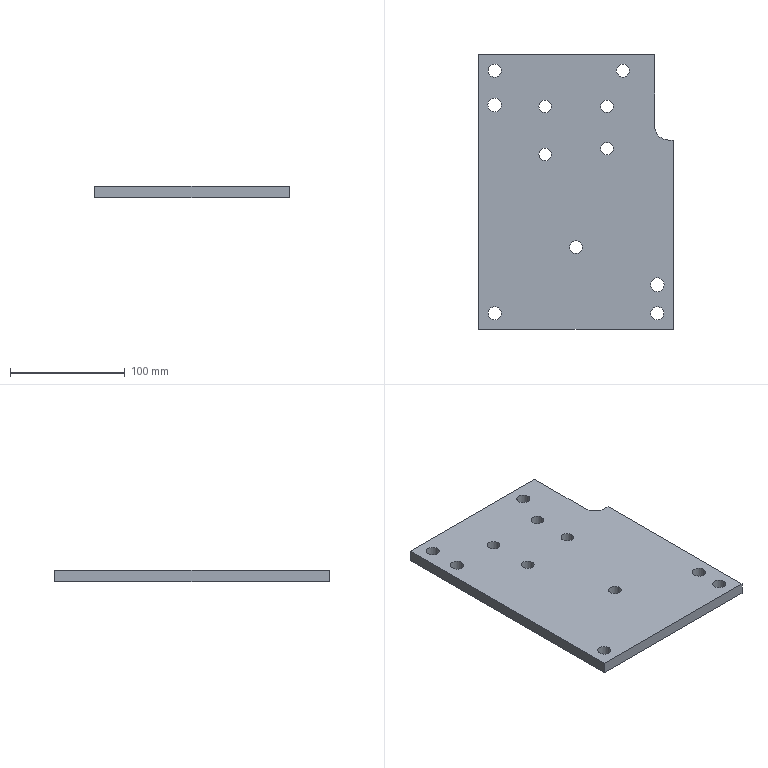Part | STEP file | lll_id2998_x_t | 1 solid | 20 faces | box 170 x 240 x 10 mm | volume 385001 mm3 | cylinder 12 | plane 8 | commonest cylinder face diameters 11 x5 11.509 x4 12 x2 24 x1
STEP:
#1=CARTESIAN_POINT('',(3581.734,-202.95,92.5));
#2=VERTEX_POINT('',#1);
#3=CARTESIAN_POINT('',(3587.234,-202.95,92.5));
#4=DIRECTION('',(0.,0.,-1.));
#5=DIRECTION('',(-1.,0.,0.));
#6=AXIS2_PLACEMENT_3D('',#3,#4,#5);
#7=CIRCLE('',#6,5.5);
#8=EDGE_CURVE('',#2,#2,#7,.T.);
#9=ORIENTED_EDGE('',*,*,#8,.F.);
#10=EDGE_LOOP('',(#9));
#11=FACE_BOUND('',#10,.T.);
#12=CARTESIAN_POINT('',(3554.876,-80.05,92.5));
#13=VERTEX_POINT('',#12);
#14=CARTESIAN_POINT('',(3560.376,-80.05,92.5));
#15=DIRECTION('',(0.,0.,1.));
#16=DIRECTION('',(-1.,0.,0.));
#17=AXIS2_PLACEMENT_3D('',#14,#15,#16);
#18=CIRCLE('',#17,5.5);
#19=EDGE_CURVE('',#13,#13,#18,.T.);
#20=ORIENTED_EDGE('',*,*,#19,.T.);
#21=EDGE_LOOP('',(#20));
#22=FACE_BOUND('',#21,.T.);
#23=CARTESIAN_POINT('',(3608.779,-80.031,92.5));
#24=VERTEX_POINT('',#23);
#25=CARTESIAN_POINT('',(3614.279,-80.031,92.5));
#26=DIRECTION('',(0.,0.,1.));
#27=DIRECTION('',(-1.,0.,0.));
#28=AXIS2_PLACEMENT_3D('',#25,#26,#27);
#29=CIRCLE('',#28,5.5);
#30=EDGE_CURVE('',#24,#24,#29,.T.);
#31=ORIENTED_EDGE('',*,*,#30,.T.);
#32=EDGE_LOOP('',(#31));
#33=FACE_BOUND('',#32,.T.);
#34=CARTESIAN_POINT('',(3510.243,-78.803,92.5));
#35=VERTEX_POINT('',#34);
#36=CARTESIAN_POINT('',(3516.243,-78.803,92.5));
#37=DIRECTION('',(0.,0.,-1.));
#38=DIRECTION('',(-1.,0.,0.));
#39=AXIS2_PLACEMENT_3D('',#36,#37,#38);
#40=CIRCLE('',#39,6.);
#41=EDGE_CURVE('',#35,#35,#40,.T.);
#42=ORIENTED_EDGE('',*,*,#41,.F.);
#43=EDGE_LOOP('',(#42));
#44=FACE_BOUND('',#43,.T.);
#45=CARTESIAN_POINT('',(3622.489,-48.803,92.5));
#46=VERTEX_POINT('',#45);
#47=CARTESIAN_POINT('',(3628.243,-48.803,92.5));
#48=DIRECTION('',(0.,0.,-1.));
#49=DIRECTION('',(-1.,0.,0.));
#50=AXIS2_PLACEMENT_3D('',#47,#48,#49);
#51=CIRCLE('',#50,5.755);
#52=EDGE_CURVE('',#46,#46,#51,.T.);
#53=ORIENTED_EDGE('',*,*,#52,.F.);
#54=EDGE_LOOP('',(#53));
#55=FACE_BOUND('',#54,.T.);
#56=CARTESIAN_POINT('',(3510.489,-48.803,92.5));
#57=VERTEX_POINT('',#56);
#58=CARTESIAN_POINT('',(3516.243,-48.803,92.5));
#59=DIRECTION('',(0.,0.,-1.));
#60=DIRECTION('',(-1.,0.,0.));
#61=AXIS2_PLACEMENT_3D('',#58,#59,#60);
#62=CIRCLE('',#61,5.755);
#63=EDGE_CURVE('',#57,#57,#62,.T.);
#64=ORIENTED_EDGE('',*,*,#63,.F.);
#65=EDGE_LOOP('',(#64));
#66=FACE_BOUND('',#65,.T.);
#67=CARTESIAN_POINT('',(3652.489,-260.803,92.5));
#68=VERTEX_POINT('',#67);
#69=CARTESIAN_POINT('',(3658.243,-260.803,92.5));
#70=DIRECTION('',(0.,0.,-1.));
#71=DIRECTION('',(-1.,0.,0.));
#72=AXIS2_PLACEMENT_3D('',#69,#70,#71);
#73=CIRCLE('',#72,5.755);
#74=EDGE_CURVE('',#68,#68,#73,.T.);
#75=ORIENTED_EDGE('',*,*,#74,.F.);
#76=EDGE_LOOP('',(#75));
#77=FACE_BOUND('',#76,.T.);
#78=CARTESIAN_POINT('',(3510.489,-260.803,92.5));
#79=VERTEX_POINT('',#78);
#80=CARTESIAN_POINT('',(3516.243,-260.803,92.5));
#81=DIRECTION('',(0.,0.,-1.));
#82=DIRECTION('',(-1.,0.,0.));
#83=AXIS2_PLACEMENT_3D('',#80,#81,#82);
#84=CIRCLE('',#83,5.755);
#85=EDGE_CURVE('',#79,#79,#84,.T.);
#86=ORIENTED_EDGE('',*,*,#85,.F.);
#87=EDGE_LOOP('',(#86));
#88=FACE_BOUND('',#87,.T.);
#89=CARTESIAN_POINT('',(3652.243,-235.803,92.5));
#90=VERTEX_POINT('',#89);
#91=CARTESIAN_POINT('',(3658.243,-235.803,92.5));
#92=DIRECTION('',(0.,0.,-1.));
#93=DIRECTION('',(-1.,0.,0.));
#94=AXIS2_PLACEMENT_3D('',#91,#92,#93);
#95=CIRCLE('',#94,6.);
#96=EDGE_CURVE('',#90,#90,#95,.T.);
#97=ORIENTED_EDGE('',*,*,#96,.F.);
#98=EDGE_LOOP('',(#97));
#99=FACE_BOUND('',#98,.T.);
#100=CARTESIAN_POINT('',(3672.243,-109.5,92.5));
#101=VERTEX_POINT('',#100);
#102=CARTESIAN_POINT('',(3668.,-109.5,92.5));
#103=VERTEX_POINT('',#102);
#104=CARTESIAN_POINT('',(3587.243,-109.5,92.5));
#105=DIRECTION('',(-1.,0.,0.));
#106=VECTOR('',#105,1.);
#107=LINE('',#104,#106);
#108=EDGE_CURVE('',#101,#103,#107,.T.);
#109=ORIENTED_EDGE('',*,*,#108,.F.);
#110=CARTESIAN_POINT('',(3672.243,-274.803,92.5));
#111=VERTEX_POINT('',#110);
#112=CARTESIAN_POINT('',(3672.243,-156.803,92.5));
#113=DIRECTION('',(0.,-1.,0.));
#114=VECTOR('',#113,1.);
#115=LINE('',#112,#114);
#116=EDGE_CURVE('',#101,#111,#115,.T.);
#117=ORIENTED_EDGE('',*,*,#116,.T.);
#118=CARTESIAN_POINT('',(3502.243,-274.803,92.5));
#119=VERTEX_POINT('',#118);
#120=CARTESIAN_POINT('',(3587.243,-274.803,92.5));
#121=DIRECTION('',(-1.,0.,0.));
#122=VECTOR('',#121,1.);
#123=LINE('',#120,#122);
#124=EDGE_CURVE('',#111,#119,#123,.T.);
#125=ORIENTED_EDGE('',*,*,#124,.T.);
#126=CARTESIAN_POINT('',(3502.243,-34.803,92.5));
#127=VERTEX_POINT('',#126);
#128=CARTESIAN_POINT('',(3502.243,-156.803,92.5));
#129=DIRECTION('',(0.,1.,0.));
#130=VECTOR('',#129,1.);
#131=LINE('',#128,#130);
#132=EDGE_CURVE('',#119,#127,#131,.T.);
#133=ORIENTED_EDGE('',*,*,#132,.T.);
#134=CARTESIAN_POINT('',(3656.,-34.803,92.5));
#135=VERTEX_POINT('',#134);
#136=CARTESIAN_POINT('',(3587.243,-34.803,92.5));
#137=DIRECTION('',(1.,0.,0.));
#138=VECTOR('',#137,1.);
#139=LINE('',#136,#138);
#140=EDGE_CURVE('',#127,#135,#139,.T.);
#141=ORIENTED_EDGE('',*,*,#140,.T.);
#142=CARTESIAN_POINT('',(3656.,-97.5,92.5));
#143=VERTEX_POINT('',#142);
#144=CARTESIAN_POINT('',(3656.,-156.803,92.5));
#145=DIRECTION('',(0.,1.,0.));
#146=VECTOR('',#145,1.);
#147=LINE('',#144,#146);
#148=EDGE_CURVE('',#143,#135,#147,.T.);
#149=ORIENTED_EDGE('',*,*,#148,.F.);
#150=CARTESIAN_POINT('',(3668.,-97.5,92.5));
#151=DIRECTION('',(0.,0.,1.));
#152=DIRECTION('',(-1.,0.,0.));
#153=AXIS2_PLACEMENT_3D('',#150,#151,#152);
#154=CIRCLE('',#153,12.);
#155=EDGE_CURVE('',#143,#103,#154,.T.);
#156=ORIENTED_EDGE('',*,*,#155,.T.);
#157=EDGE_LOOP('',(#109,#117,#125,#133,#141,#149,#156));
#158=FACE_BOUND('',#157,.T.);
#159=CARTESIAN_POINT('',(3608.779,-117.031,92.5));
#160=VERTEX_POINT('',#159);
#161=CARTESIAN_POINT('',(3614.279,-117.031,92.5));
#162=DIRECTION('',(0.,0.,1.));
#163=DIRECTION('',(-1.,0.,0.));
#164=AXIS2_PLACEMENT_3D('',#161,#162,#163);
#165=CIRCLE('',#164,5.5);
#166=EDGE_CURVE('',#160,#160,#165,.T.);
#167=ORIENTED_EDGE('',*,*,#166,.T.);
#168=EDGE_LOOP('',(#167));
#169=FACE_BOUND('',#168,.T.);
#170=CARTESIAN_POINT('',(3554.876,-122.05,92.5));
#171=VERTEX_POINT('',#170);
#172=CARTESIAN_POINT('',(3560.376,-122.05,92.5));
#173=DIRECTION('',(0.,0.,1.));
#174=DIRECTION('',(-1.,0.,0.));
#175=AXIS2_PLACEMENT_3D('',#172,#173,#174);
#176=CIRCLE('',#175,5.5);
#177=EDGE_CURVE('',#171,#171,#176,.T.);
#178=ORIENTED_EDGE('',*,*,#177,.T.);
#179=EDGE_LOOP('',(#178));
#180=FACE_BOUND('',#179,.T.);
#181=CARTESIAN_POINT('',(3587.243,-156.803,92.5));
#182=DIRECTION('',(0.,0.,-1.));
#183=DIRECTION('',(1.,0.,0.));
#184=AXIS2_PLACEMENT_3D('',#181,#182,#183);
#185=PLANE('',#184);
#186=ADVANCED_FACE('',(#11,#22,#33,#44,#55,#66,#77,#88,#99,#158,#169,#180),#185,.T.);
#187=CARTESIAN_POINT('',(3581.734,-202.95,102.5));
#188=VERTEX_POINT('',#187);
#189=CARTESIAN_POINT('',(3587.234,-202.95,102.5));
#190=DIRECTION('',(0.,0.,-1.));
#191=DIRECTION('',(-1.,0.,0.));
#192=AXIS2_PLACEMENT_3D('',#189,#190,#191);
#193=CIRCLE('',#192,5.5);
#194=EDGE_CURVE('',#188,#188,#193,.T.);
#195=ORIENTED_EDGE('',*,*,#194,.T.);
#196=EDGE_LOOP('',(#195));
#197=FACE_BOUND('',#196,.T.);
#198=CARTESIAN_POINT('',(3554.876,-80.05,102.5));
#199=VERTEX_POINT('',#198);
#200=CARTESIAN_POINT('',(3560.376,-80.05,102.5));
#201=DIRECTION('',(0.,0.,1.));
#202=DIRECTION('',(-1.,0.,0.));
#203=AXIS2_PLACEMENT_3D('',#200,#201,#202);
#204=CIRCLE('',#203,5.5);
#205=EDGE_CURVE('',#199,#199,#204,.T.);
#206=ORIENTED_EDGE('',*,*,#205,.F.);
#207=EDGE_LOOP('',(#206));
#208=FACE_BOUND('',#207,.T.);
#209=CARTESIAN_POINT('',(3608.779,-80.031,102.5));
#210=VERTEX_POINT('',#209);
#211=CARTESIAN_POINT('',(3614.279,-80.031,102.5));
#212=DIRECTION('',(0.,0.,1.));
#213=DIRECTION('',(-1.,0.,0.));
#214=AXIS2_PLACEMENT_3D('',#211,#212,#213);
#215=CIRCLE('',#214,5.5);
#216=EDGE_CURVE('',#210,#210,#215,.T.);
#217=ORIENTED_EDGE('',*,*,#216,.F.);
#218=EDGE_LOOP('',(#217));
#219=FACE_BOUND('',#218,.T.);
#220=CARTESIAN_POINT('',(3510.489,-48.803,102.5));
#221=VERTEX_POINT('',#220);
#222=CARTESIAN_POINT('',(3516.243,-48.803,102.5));
#223=DIRECTION('',(0.,0.,1.));
#224=DIRECTION('',(-1.,0.,0.));
#225=AXIS2_PLACEMENT_3D('',#222,#223,#224);
#226=CIRCLE('',#225,5.755);
#227=EDGE_CURVE('',#221,#221,#226,.T.);
#228=ORIENTED_EDGE('',*,*,#227,.F.);
#229=EDGE_LOOP('',(#228));
#230=FACE_BOUND('',#229,.T.);
#231=CARTESIAN_POINT('',(3622.489,-48.803,102.5));
#232=VERTEX_POINT('',#231);
#233=CARTESIAN_POINT('',(3628.243,-48.803,102.5));
#234=DIRECTION('',(0.,0.,-1.));
#235=DIRECTION('',(-1.,0.,0.));
#236=AXIS2_PLACEMENT_3D('',#233,#234,#235);
#237=CIRCLE('',#236,5.755);
#238=EDGE_CURVE('',#232,#232,#237,.T.);
#239=ORIENTED_EDGE('',*,*,#238,.T.);
#240=EDGE_LOOP('',(#239));
#241=FACE_BOUND('',#240,.T.);
#242=CARTESIAN_POINT('',(3510.243,-78.803,102.5));
#243=VERTEX_POINT('',#242);
#244=CARTESIAN_POINT('',(3516.243,-78.803,102.5));
#245=DIRECTION('',(0.,0.,-1.));
#246=DIRECTION('',(-1.,0.,0.));
#247=AXIS2_PLACEMENT_3D('',#244,#245,#246);
#248=CIRCLE('',#247,6.);
#249=EDGE_CURVE('',#243,#243,#248,.T.);
#250=ORIENTED_EDGE('',*,*,#249,.T.);
#251=EDGE_LOOP('',(#250));
#252=FACE_BOUND('',#251,.T.);
#253=CARTESIAN_POINT('',(3502.243,-274.803,102.5));
#254=VERTEX_POINT('',#253);
#255=CARTESIAN_POINT('',(3672.243,-274.803,102.5));
#256=VERTEX_POINT('',#255);
#257=CARTESIAN_POINT('',(3587.243,-274.803,102.5));
#258=DIRECTION('',(1.,0.,0.));
#259=VECTOR('',#258,1.);
#260=LINE('',#257,#259);
#261=EDGE_CURVE('',#254,#256,#260,.T.);
#262=ORIENTED_EDGE('',*,*,#261,.T.);
#263=CARTESIAN_POINT('',(3672.243,-109.5,102.5));
#264=VERTEX_POINT('',#263);
#265=CARTESIAN_POINT('',(3672.243,-156.803,102.5));
#266=DIRECTION('',(0.,1.,0.));
#267=VECTOR('',#266,1.);
#268=LINE('',#265,#267);
#269=EDGE_CURVE('',#256,#264,#268,.T.);
#270=ORIENTED_EDGE('',*,*,#269,.T.);
#271=CARTESIAN_POINT('',(3668.,-109.5,102.5));
#272=VERTEX_POINT('',#271);
#273=CARTESIAN_POINT('',(3312.867,-109.5,102.5));
#274=DIRECTION('',(-1.,0.,0.));
#275=VECTOR('',#274,1.);
#276=LINE('',#273,#275);
#277=EDGE_CURVE('',#264,#272,#276,.T.);
#278=ORIENTED_EDGE('',*,*,#277,.T.);
#279=CARTESIAN_POINT('',(3656.,-97.5,102.5));
#280=VERTEX_POINT('',#279);
#281=CARTESIAN_POINT('',(3668.,-97.5,102.5));
#282=DIRECTION('',(0.,0.,1.));
#283=DIRECTION('',(-1.,0.,0.));
#284=AXIS2_PLACEMENT_3D('',#281,#282,#283);
#285=CIRCLE('',#284,12.);
#286=EDGE_CURVE('',#280,#272,#285,.T.);
#287=ORIENTED_EDGE('',*,*,#286,.F.);
#288=CARTESIAN_POINT('',(3656.,-34.803,102.5));
#289=VERTEX_POINT('',#288);
#290=CARTESIAN_POINT('',(3656.,136.288,102.5));
#291=DIRECTION('',(0.,1.,0.));
#292=VECTOR('',#291,1.);
#293=LINE('',#290,#292);
#294=EDGE_CURVE('',#280,#289,#293,.T.);
#295=ORIENTED_EDGE('',*,*,#294,.T.);
#296=CARTESIAN_POINT('',(3502.243,-34.803,102.5));
#297=VERTEX_POINT('',#296);
#298=CARTESIAN_POINT('',(3587.243,-34.803,102.5));
#299=DIRECTION('',(1.,0.,0.));
#300=VECTOR('',#299,1.);
#301=LINE('',#298,#300);
#302=EDGE_CURVE('',#297,#289,#301,.T.);
#303=ORIENTED_EDGE('',*,*,#302,.F.);
#304=CARTESIAN_POINT('',(3502.243,-156.803,102.5));
#305=DIRECTION('',(0.,1.,0.));
#306=VECTOR('',#305,1.);
#307=LINE('',#304,#306);
#308=EDGE_CURVE('',#254,#297,#307,.T.);
#309=ORIENTED_EDGE('',*,*,#308,.F.);
#310=EDGE_LOOP('',(#262,#270,#278,#287,#295,#303,#309));
#311=FACE_BOUND('',#310,.T.);
#312=CARTESIAN_POINT('',(3652.243,-235.803,102.5));
#313=VERTEX_POINT('',#312);
#314=CARTESIAN_POINT('',(3658.243,-235.803,102.5));
#315=DIRECTION('',(0.,0.,1.));
#316=DIRECTION('',(-1.,0.,0.));
#317=AXIS2_PLACEMENT_3D('',#314,#315,#316);
#318=CIRCLE('',#317,6.);
#319=EDGE_CURVE('',#313,#313,#318,.T.);
#320=ORIENTED_EDGE('',*,*,#319,.F.);
#321=EDGE_LOOP('',(#320));
#322=FACE_BOUND('',#321,.T.);
#323=CARTESIAN_POINT('',(3510.489,-260.803,102.5));
#324=VERTEX_POINT('',#323);
#325=CARTESIAN_POINT('',(3516.243,-260.803,102.5));
#326=DIRECTION('',(0.,0.,1.));
#327=DIRECTION('',(-1.,0.,0.));
#328=AXIS2_PLACEMENT_3D('',#325,#326,#327);
#329=CIRCLE('',#328,5.755);
#330=EDGE_CURVE('',#324,#324,#329,.T.);
#331=ORIENTED_EDGE('',*,*,#330,.F.);
#332=EDGE_LOOP('',(#331));
#333=FACE_BOUND('',#332,.T.);
#334=CARTESIAN_POINT('',(3652.489,-260.803,102.5));
#335=VERTEX_POINT('',#334);
#336=CARTESIAN_POINT('',(3658.243,-260.803,102.5));
#337=DIRECTION('',(0.,0.,-1.));
#338=DIRECTION('',(-1.,0.,0.));
#339=AXIS2_PLACEMENT_3D('',#336,#337,#338);
#340=CIRCLE('',#339,5.755);
#341=EDGE_CURVE('',#335,#335,#340,.T.);
#342=ORIENTED_EDGE('',*,*,#341,.T.);
#343=EDGE_LOOP('',(#342));
#344=FACE_BOUND('',#343,.T.);
#345=CARTESIAN_POINT('',(3608.779,-117.031,102.5));
#346=VERTEX_POINT('',#345);
#347=CARTESIAN_POINT('',(3614.279,-117.031,102.5));
#348=DIRECTION('',(0.,0.,1.));
#349=DIRECTION('',(-1.,0.,0.));
#350=AXIS2_PLACEMENT_3D('',#347,#348,#349);
#351=CIRCLE('',#350,5.5);
#352=EDGE_CURVE('',#346,#346,#351,.T.);
#353=ORIENTED_EDGE('',*,*,#352,.F.);
#354=EDGE_LOOP('',(#353));
#355=FACE_BOUND('',#354,.T.);
#356=CARTESIAN_POINT('',(3554.876,-122.05,102.5));
#357=VERTEX_POINT('',#356);
#358=CARTESIAN_POINT('',(3560.376,-122.05,102.5));
#359=DIRECTION('',(0.,0.,1.));
#360=DIRECTION('',(-1.,0.,0.));
#361=AXIS2_PLACEMENT_3D('',#358,#359,#360);
#362=CIRCLE('',#361,5.5);
#363=EDGE_CURVE('',#357,#357,#362,.T.);
#364=ORIENTED_EDGE('',*,*,#363,.F.);
#365=EDGE_LOOP('',(#364));
#366=FACE_BOUND('',#365,.T.);
#367=CARTESIAN_POINT('',(3312.867,136.288,102.5));
#368=DIRECTION('',(0.,0.,-1.));
#369=DIRECTION('',(-1.,0.,0.));
#370=AXIS2_PLACEMENT_3D('',#367,#368,#369);
#371=PLANE('',#370);
#372=ADVANCED_FACE('',(#197,#208,#219,#230,#241,#252,#311,#322,#333,#344,#355,#366),#371,.F.);
#373=ORIENTED_EDGE('',*,*,#319,.T.);
#374=EDGE_LOOP('',(#373));
#375=FACE_BOUND('',#374,.T.);
#376=ORIENTED_EDGE('',*,*,#96,.T.);
#377=EDGE_LOOP('',(#376));
#378=FACE_BOUND('',#377,.T.);
#379=CARTESIAN_POINT('',(3658.243,-235.803,92.5));
#380=DIRECTION('',(0.,0.,1.));
#381=DIRECTION('',(-1.,0.,0.));
#382=AXIS2_PLACEMENT_3D('',#379,#380,#381);
#383=CYLINDRICAL_SURFACE('',#382,6.);
#384=ADVANCED_FACE('',(#375,#378),#383,.F.);
#385=ORIENTED_EDGE('',*,*,#330,.T.);
#386=EDGE_LOOP('',(#385));
#387=FACE_BOUND('',#386,.T.);
#388=ORIENTED_EDGE('',*,*,#85,.T.);
#389=EDGE_LOOP('',(#388));
#390=FACE_BOUND('',#389,.T.);
#391=CARTESIAN_POINT('',(3516.243,-260.803,92.5));
#392=DIRECTION('',(0.,0.,1.));
#393=DIRECTION('',(-1.,0.,0.));
#394=AXIS2_PLACEMENT_3D('',#391,#392,#393);
#395=CYLINDRICAL_SURFACE('',#394,5.755);
#396=ADVANCED_FACE('',(#387,#390),#395,.F.);
#397=ORIENTED_EDGE('',*,*,#341,.F.);
#398=EDGE_LOOP('',(#397));
#399=FACE_BOUND('',#398,.T.);
#400=ORIENTED_EDGE('',*,*,#74,.T.);
#401=EDGE_LOOP('',(#400));
#402=FACE_BOUND('',#401,.T.);
#403=CARTESIAN_POINT('',(3658.243,-260.803,92.5));
#404=DIRECTION('',(0.,0.,1.));
#405=DIRECTION('',(-1.,0.,0.));
#406=AXIS2_PLACEMENT_3D('',#403,#404,#405);
#407=CYLINDRICAL_SURFACE('',#406,5.755);
#408=ADVANCED_FACE('',(#399,#402),#407,.F.);
#409=ORIENTED_EDGE('',*,*,#227,.T.);
#410=EDGE_LOOP('',(#409));
#411=FACE_BOUND('',#410,.T.);
#412=ORIENTED_EDGE('',*,*,#63,.T.);
#413=EDGE_LOOP('',(#412));
#414=FACE_BOUND('',#413,.T.);
#415=CARTESIAN_POINT('',(3516.243,-48.803,92.5));
#416=DIRECTION('',(0.,0.,1.));
#417=DIRECTION('',(-1.,0.,0.));
#418=AXIS2_PLACEMENT_3D('',#415,#416,#417);
#419=CYLINDRICAL_SURFACE('',#418,5.755);
#420=ADVANCED_FACE('',(#411,#414),#419,.F.);
#421=ORIENTED_EDGE('',*,*,#238,.F.);
#422=EDGE_LOOP('',(#421));
#423=FACE_BOUND('',#422,.T.);
#424=ORIENTED_EDGE('',*,*,#52,.T.);
#425=EDGE_LOOP('',(#424));
#426=FACE_BOUND('',#425,.T.);
#427=CARTESIAN_POINT('',(3628.243,-48.803,92.5));
#428=DIRECTION('',(0.,0.,1.));
#429=DIRECTION('',(-1.,0.,0.));
#430=AXIS2_PLACEMENT_3D('',#427,#428,#429);
#431=CYLINDRICAL_SURFACE('',#430,5.755);
#432=ADVANCED_FACE('',(#423,#426),#431,.F.);
#433=ORIENTED_EDGE('',*,*,#249,.F.);
#434=EDGE_LOOP('',(#433));
#435=FACE_BOUND('',#434,.T.);
#436=ORIENTED_EDGE('',*,*,#41,.T.);
#437=EDGE_LOOP('',(#436));
#438=FACE_BOUND('',#437,.T.);
#439=CARTESIAN_POINT('',(3516.243,-78.803,92.5));
#440=DIRECTION('',(0.,0.,1.));
#441=DIRECTION('',(-1.,0.,0.));
#442=AXIS2_PLACEMENT_3D('',#439,#440,#441);
#443=CYLINDRICAL_SURFACE('',#442,6.);
#444=ADVANCED_FACE('',(#435,#438),#443,.F.);
#445=ORIENTED_EDGE('',*,*,#308,.T.);
#446=CARTESIAN_POINT('',(3502.243,-34.803,92.5));
#447=DIRECTION('',(0.,0.,1.));
#448=VECTOR('',#447,1.);
#449=LINE('',#446,#448);
#450=EDGE_CURVE('',#127,#297,#449,.T.);
#451=ORIENTED_EDGE('',*,*,#450,.F.);
#452=ORIENTED_EDGE('',*,*,#132,.F.);
#453=CARTESIAN_POINT('',(3502.243,-274.803,92.5));
#454=DIRECTION('',(0.,0.,1.));
#455=VECTOR('',#454,1.);
#456=LINE('',#453,#455);
#457=EDGE_CURVE('',#119,#254,#456,.T.);
#458=ORIENTED_EDGE('',*,*,#457,.T.);
#459=EDGE_LOOP('',(#445,#451,#452,#458));
#460=FACE_OUTER_BOUND('',#459,.T.);
#461=CARTESIAN_POINT('',(3502.243,-156.803,92.5));
#462=DIRECTION('',(-1.,0.,0.));
#463=DIRECTION('',(0.,0.,-1.));
#464=AXIS2_PLACEMENT_3D('',#461,#462,#463);
#465=PLANE('',#464);
#466=ADVANCED_FACE('',(#460),#465,.T.);
#467=CARTESIAN_POINT('',(3656.,-97.5,60.5));
#468=DIRECTION('',(0.,0.,-1.));
#469=VECTOR('',#468,1.);
#470=LINE('',#467,#469);
#471=EDGE_CURVE('',#280,#143,#470,.T.);
#472=ORIENTED_EDGE('',*,*,#471,.F.);
#473=ORIENTED_EDGE('',*,*,#286,.T.);
#474=CARTESIAN_POINT('',(3668.,-109.5,60.5));
#475=DIRECTION('',(0.,0.,1.));
#476=VECTOR('',#475,1.);
#477=LINE('',#474,#476);
#478=EDGE_CURVE('',#103,#272,#477,.T.);
#479=ORIENTED_EDGE('',*,*,#478,.F.);
#480=ORIENTED_EDGE('',*,*,#155,.F.);
#481=EDGE_LOOP('',(#472,#473,#479,#480));
#482=FACE_OUTER_BOUND('',#481,.T.);
#483=CARTESIAN_POINT('',(3668.,-97.5,60.5));
#484=DIRECTION('',(0.,0.,-1.));
#485=DIRECTION('',(-1.,0.,0.));
#486=AXIS2_PLACEMENT_3D('',#483,#484,#485);
#487=CYLINDRICAL_SURFACE('',#486,12.);
#488=ADVANCED_FACE('',(#482),#487,.F.);
#489=ORIENTED_EDGE('',*,*,#478,.T.);
#490=ORIENTED_EDGE('',*,*,#277,.F.);
#491=CARTESIAN_POINT('',(3672.243,-109.5,60.5));
#492=DIRECTION('',(0.,0.,1.));
#493=VECTOR('',#492,1.);
#494=LINE('',#491,#493);
#495=EDGE_CURVE('',#101,#264,#494,.T.);
#496=ORIENTED_EDGE('',*,*,#495,.F.);
#497=ORIENTED_EDGE('',*,*,#108,.T.);
#498=EDGE_LOOP('',(#489,#490,#496,#497));
#499=FACE_OUTER_BOUND('',#498,.T.);
#500=CARTESIAN_POINT('',(3700.5,-109.5,60.5));
#501=DIRECTION('',(0.,-1.,0.));
#502=DIRECTION('',(0.,0.,1.));
#503=AXIS2_PLACEMENT_3D('',#500,#501,#502);
#504=PLANE('',#503);
#505=ADVANCED_FACE('',(#499),#504,.F.);
#506=CARTESIAN_POINT('',(3656.,-34.803,60.5));
#507=DIRECTION('',(0.,0.,-1.));
#508=VECTOR('',#507,1.);
#509=LINE('',#506,#508);
#510=EDGE_CURVE('',#289,#135,#509,.T.);
#511=ORIENTED_EDGE('',*,*,#510,.F.);
#512=ORIENTED_EDGE('',*,*,#294,.F.);
#513=ORIENTED_EDGE('',*,*,#471,.T.);
#514=ORIENTED_EDGE('',*,*,#148,.T.);
#515=EDGE_LOOP('',(#511,#512,#513,#514));
#516=FACE_OUTER_BOUND('',#515,.T.);
#517=CARTESIAN_POINT('',(3656.,0.00007612,60.5));
#518=DIRECTION('',(-1.,0.,0.));
#519=DIRECTION('',(0.,0.,-1.));
#520=AXIS2_PLACEMENT_3D('',#517,#518,#519);
#521=PLANE('',#520);
#522=ADVANCED_FACE('',(#516),#521,.F.);
#523=ORIENTED_EDGE('',*,*,#302,.T.);
#524=ORIENTED_EDGE('',*,*,#510,.T.);
#525=ORIENTED_EDGE('',*,*,#140,.F.);
#526=ORIENTED_EDGE('',*,*,#450,.T.);
#527=EDGE_LOOP('',(#523,#524,#525,#526));
#528=FACE_OUTER_BOUND('',#527,.T.);
#529=CARTESIAN_POINT('',(3587.243,-34.803,92.5));
#530=DIRECTION('',(0.,1.,0.));
#531=DIRECTION('',(0.,0.,1.));
#532=AXIS2_PLACEMENT_3D('',#529,#530,#531);
#533=PLANE('',#532);
#534=ADVANCED_FACE('',(#528),#533,.T.);
#535=ORIENTED_EDGE('',*,*,#261,.F.);
#536=ORIENTED_EDGE('',*,*,#457,.F.);
#537=ORIENTED_EDGE('',*,*,#124,.F.);
#538=CARTESIAN_POINT('',(3672.243,-274.803,92.5));
#539=DIRECTION('',(0.,0.,1.));
#540=VECTOR('',#539,1.);
#541=LINE('',#538,#540);
#542=EDGE_CURVE('',#111,#256,#541,.T.);
#543=ORIENTED_EDGE('',*,*,#542,.T.);
#544=EDGE_LOOP('',(#535,#536,#537,#543));
#545=FACE_OUTER_BOUND('',#544,.T.);
#546=CARTESIAN_POINT('',(3587.243,-274.803,92.5));
#547=DIRECTION('',(0.,-1.,0.));
#548=DIRECTION('',(0.,0.,-1.));
#549=AXIS2_PLACEMENT_3D('',#546,#547,#548);
#550=PLANE('',#549);
#551=ADVANCED_FACE('',(#545),#550,.T.);
#552=ORIENTED_EDGE('',*,*,#269,.F.);
#553=ORIENTED_EDGE('',*,*,#542,.F.);
#554=ORIENTED_EDGE('',*,*,#116,.F.);
#555=ORIENTED_EDGE('',*,*,#495,.T.);
#556=EDGE_LOOP('',(#552,#553,#554,#555));
#557=FACE_OUTER_BOUND('',#556,.T.);
#558=CARTESIAN_POINT('',(3672.243,-156.803,92.5));
#559=DIRECTION('',(1.,0.,0.));
#560=DIRECTION('',(0.,0.,1.));
#561=AXIS2_PLACEMENT_3D('',#558,#559,#560);
#562=PLANE('',#561);
#563=ADVANCED_FACE('',(#557),#562,.T.);
#564=ORIENTED_EDGE('',*,*,#30,.F.);
#565=EDGE_LOOP('',(#564));
#566=FACE_BOUND('',#565,.T.);
#567=ORIENTED_EDGE('',*,*,#216,.T.);
#568=EDGE_LOOP('',(#567));
#569=FACE_BOUND('',#568,.T.);
#570=CARTESIAN_POINT('',(3614.279,-80.031,212.5));
#571=DIRECTION('',(0.,0.,-1.));
#572=DIRECTION('',(-1.,0.,0.));
#573=AXIS2_PLACEMENT_3D('',#570,#571,#572);
#574=CYLINDRICAL_SURFACE('',#573,5.5);
#575=ADVANCED_FACE('',(#566,#569),#574,.F.);
#576=ORIENTED_EDGE('',*,*,#166,.F.);
#577=EDGE_LOOP('',(#576));
#578=FACE_BOUND('',#577,.T.);
#579=ORIENTED_EDGE('',*,*,#352,.T.);
#580=EDGE_LOOP('',(#579));
#581=FACE_BOUND('',#580,.T.);
#582=CARTESIAN_POINT('',(3614.279,-117.031,212.5));
#583=DIRECTION('',(0.,0.,-1.));
#584=DIRECTION('',(-1.,0.,0.));
#585=AXIS2_PLACEMENT_3D('',#582,#583,#584);
#586=CYLINDRICAL_SURFACE('',#585,5.5);
#587=ADVANCED_FACE('',(#578,#581),#586,.F.);
#588=ORIENTED_EDGE('',*,*,#19,.F.);
#589=EDGE_LOOP('',(#588));
#590=FACE_BOUND('',#589,.T.);
#591=ORIENTED_EDGE('',*,*,#205,.T.);
#592=EDGE_LOOP('',(#591));
#593=FACE_BOUND('',#592,.T.);
#594=CARTESIAN_POINT('',(3560.376,-80.05,212.5));
#595=DIRECTION('',(0.,0.,-1.));
#596=DIRECTION('',(-1.,0.,0.));
#597=AXIS2_PLACEMENT_3D('',#594,#595,#596);
#598=CYLINDRICAL_SURFACE('',#597,5.5);
#599=ADVANCED_FACE('',(#590,#593),#598,.F.);
#600=ORIENTED_EDGE('',*,*,#177,.F.);
#601=EDGE_LOOP('',(#600));
#602=FACE_BOUND('',#601,.T.);
#603=ORIENTED_EDGE('',*,*,#363,.T.);
#604=EDGE_LOOP('',(#603));
#605=FACE_BOUND('',#604,.T.);
#606=CARTESIAN_POINT('',(3560.376,-122.05,212.5));
#607=DIRECTION('',(0.,0.,-1.));
#608=DIRECTION('',(-1.,0.,0.));
#609=AXIS2_PLACEMENT_3D('',#606,#607,#608);
#610=CYLINDRICAL_SURFACE('',#609,5.5);
#611=ADVANCED_FACE('',(#602,#605),#610,.F.);
#612=ORIENTED_EDGE('',*,*,#8,.T.);
#613=EDGE_LOOP('',(#612));
#614=FACE_BOUND('',#613,.T.);
#615=ORIENTED_EDGE('',*,*,#194,.F.);
#616=EDGE_LOOP('',(#615));
#617=FACE_BOUND('',#616,.T.);
#618=CARTESIAN_POINT('',(3587.234,-202.95,77.5));
#619=DIRECTION('',(0.,0.,1.));
#620=DIRECTION('',(-1.,0.,0.));
#621=AXIS2_PLACEMENT_3D('',#618,#619,#620);
#622=CYLINDRICAL_SURFACE('',#621,5.5);
#623=ADVANCED_FACE('',(#614,#617),#622,.F.);
#624=CLOSED_SHELL('',(#186,#372,#384,#396,#408,#420,#432,#444,#466,#488,#505,#522,#534,#551,#563,#575,#587,#599,#611,#623));
#625=MANIFOLD_SOLID_BREP('',#624);
#626=(LENGTH_UNIT()NAMED_UNIT(*)SI_UNIT(.MILLI.,.METRE.));
#627=UNCERTAINTY_MEASURE_WITH_UNIT(LENGTH_MEASURE(0.00002),#626,'','');
#628=(NAMED_UNIT(*)PLANE_ANGLE_UNIT()SI_UNIT($,.RADIAN.));
#629=PLANE_ANGLE_MEASURE_WITH_UNIT(PLANE_ANGLE_MEASURE(0.01745),#628);
#630=DIMENSIONAL_EXPONENTS(0.,0.,0.,0.,0.,0.,0.);
#631=(CONVERSION_BASED_UNIT('DEGREE',#629)NAMED_UNIT(#630)PLANE_ANGLE_UNIT());
#632=(NAMED_UNIT(*)SI_UNIT($,.STERADIAN.)SOLID_ANGLE_UNIT());
#633=(GEOMETRIC_REPRESENTATION_CONTEXT(3)GLOBAL_UNCERTAINTY_ASSIGNED_CONTEXT((#627))GLOBAL_UNIT_ASSIGNED_CONTEXT((#626,#631,#632))REPRESENTATION_CONTEXT('',''));
#634=ADVANCED_BREP_SHAPE_REPRESENTATION('',(#625),#633);